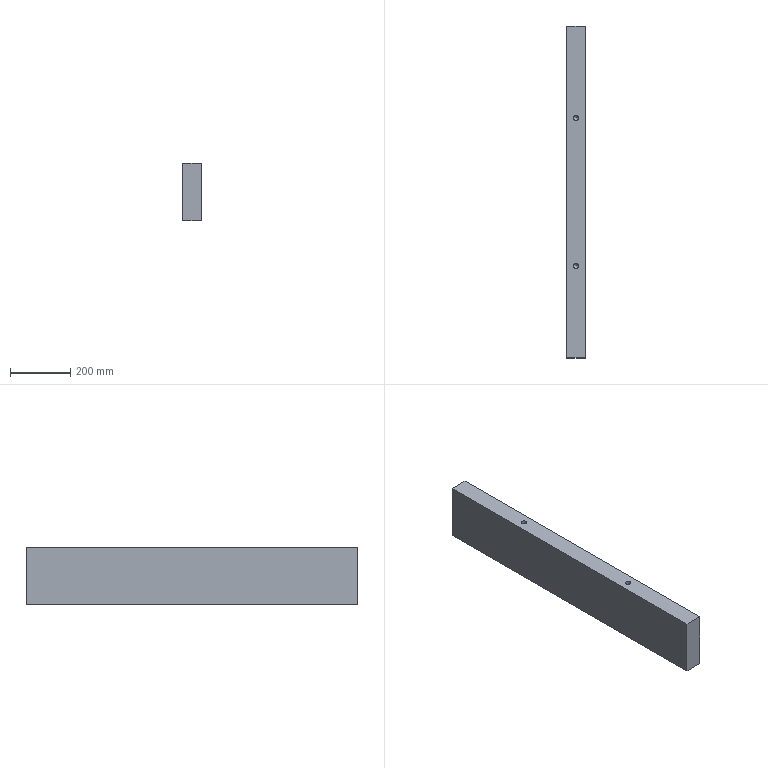Part | STEP file | lll_id4450_x_t | 1 solid | 14 faces | box 60 x 1100 x 190 mm | volume 12497474 mm3 | plane 6 | cylinder 4 | cone 4 | commonest cylinder face diameters 17.506 x4
STEP:
#1=CARTESIAN_POINT('',(2116.188,-465.,-370.));
#2=VERTEX_POINT('',#1);
#3=CARTESIAN_POINT('',(2107.435,-465.,-370.));
#4=DIRECTION('',(0.,0.,1.));
#5=DIRECTION('',(1.,0.,0.));
#6=AXIS2_PLACEMENT_3D('',#3,#4,#5);
#7=CIRCLE('',#6,8.753);
#8=EDGE_CURVE('',#2,#2,#7,.T.);
#9=ORIENTED_EDGE('',*,*,#8,.T.);
#10=EDGE_LOOP('',(#9));
#11=FACE_BOUND('',#10,.T.);
#12=CARTESIAN_POINT('',(2077.435,550.,-370.));
#13=VERTEX_POINT('',#12);
#14=CARTESIAN_POINT('',(2077.435,-550.,-370.));
#15=VERTEX_POINT('',#14);
#16=CARTESIAN_POINT('',(2077.435,1.,-370.));
#17=DIRECTION('',(0.,-1.,0.));
#18=VECTOR('',#17,1.);
#19=LINE('',#16,#18);
#20=EDGE_CURVE('',#13,#15,#19,.T.);
#21=ORIENTED_EDGE('',*,*,#20,.F.);
#22=CARTESIAN_POINT('',(2137.435,550.,-370.));
#23=VERTEX_POINT('',#22);
#24=CARTESIAN_POINT('',(4323.751,550.,-370.));
#25=DIRECTION('',(1.,0.,0.));
#26=VECTOR('',#25,1.);
#27=LINE('',#24,#26);
#28=EDGE_CURVE('',#13,#23,#27,.T.);
#29=ORIENTED_EDGE('',*,*,#28,.T.);
#30=CARTESIAN_POINT('',(2137.435,-550.,-370.));
#31=VERTEX_POINT('',#30);
#32=CARTESIAN_POINT('',(2137.435,600.,-370.));
#33=DIRECTION('',(0.,-1.,0.));
#34=VECTOR('',#33,1.);
#35=LINE('',#32,#34);
#36=EDGE_CURVE('',#23,#31,#35,.T.);
#37=ORIENTED_EDGE('',*,*,#36,.T.);
#38=CARTESIAN_POINT('',(4323.751,-550.,-370.));
#39=DIRECTION('',(-1.,0.,0.));
#40=VECTOR('',#39,1.);
#41=LINE('',#38,#40);
#42=EDGE_CURVE('',#31,#15,#41,.T.);
#43=ORIENTED_EDGE('',*,*,#42,.T.);
#44=EDGE_LOOP('',(#21,#29,#37,#43));
#45=FACE_BOUND('',#44,.T.);
#46=CARTESIAN_POINT('',(2116.188,465.,-370.));
#47=VERTEX_POINT('',#46);
#48=CARTESIAN_POINT('',(2107.435,465.,-370.));
#49=DIRECTION('',(0.,0.,1.));
#50=DIRECTION('',(1.,0.,0.));
#51=AXIS2_PLACEMENT_3D('',#48,#49,#50);
#52=CIRCLE('',#51,8.753);
#53=EDGE_CURVE('',#47,#47,#52,.T.);
#54=ORIENTED_EDGE('',*,*,#53,.T.);
#55=EDGE_LOOP('',(#54));
#56=FACE_BOUND('',#55,.T.);
#57=CARTESIAN_POINT('',(4323.751,1.,-370.));
#58=DIRECTION('',(0.,0.,-1.));
#59=DIRECTION('',(-1.,0.,0.));
#60=AXIS2_PLACEMENT_3D('',#57,#58,#59);
#61=PLANE('',#60);
#62=ADVANCED_FACE('',(#11,#45,#56),#61,.T.);
#63=ORIENTED_EDGE('',*,*,#36,.F.);
#64=CARTESIAN_POINT('',(2137.435,550.,-180.));
#65=VERTEX_POINT('',#64);
#66=CARTESIAN_POINT('',(2137.435,550.,-182.5));
#67=DIRECTION('',(0.,0.,-1.));
#68=VECTOR('',#67,1.);
#69=LINE('',#66,#68);
#70=EDGE_CURVE('',#65,#23,#69,.T.);
#71=ORIENTED_EDGE('',*,*,#70,.F.);
#72=CARTESIAN_POINT('',(2137.435,-550.,-180.));
#73=VERTEX_POINT('',#72);
#74=CARTESIAN_POINT('',(2137.435,1.,-180.));
#75=DIRECTION('',(0.,-1.,0.));
#76=VECTOR('',#75,1.);
#77=LINE('',#74,#76);
#78=EDGE_CURVE('',#65,#73,#77,.T.);
#79=ORIENTED_EDGE('',*,*,#78,.T.);
#80=CARTESIAN_POINT('',(2137.435,-550.,-182.5));
#81=DIRECTION('',(0.,0.,-1.));
#82=VECTOR('',#81,1.);
#83=LINE('',#80,#82);
#84=EDGE_CURVE('',#73,#31,#83,.T.);
#85=ORIENTED_EDGE('',*,*,#84,.T.);
#86=EDGE_LOOP('',(#63,#71,#79,#85));
#87=FACE_OUTER_BOUND('',#86,.T.);
#88=CARTESIAN_POINT('',(2137.435,600.,-182.5));
#89=DIRECTION('',(1.,0.,0.));
#90=DIRECTION('',(0.,0.,-1.));
#91=AXIS2_PLACEMENT_3D('',#88,#89,#90);
#92=PLANE('',#91);
#93=ADVANCED_FACE('',(#87),#92,.T.);
#94=CARTESIAN_POINT('',(2077.435,-550.,-180.));
#95=VERTEX_POINT('',#94);
#96=CARTESIAN_POINT('',(2077.435,-550.,-251.25));
#97=DIRECTION('',(0.,0.,-1.));
#98=VECTOR('',#97,1.);
#99=LINE('',#96,#98);
#100=EDGE_CURVE('',#95,#15,#99,.T.);
#101=ORIENTED_EDGE('',*,*,#100,.T.);
#102=ORIENTED_EDGE('',*,*,#42,.F.);
#103=ORIENTED_EDGE('',*,*,#84,.F.);
#104=CARTESIAN_POINT('',(4323.751,-550.,-180.));
#105=DIRECTION('',(-1.,0.,0.));
#106=VECTOR('',#105,1.);
#107=LINE('',#104,#106);
#108=EDGE_CURVE('',#73,#95,#107,.T.);
#109=ORIENTED_EDGE('',*,*,#108,.T.);
#110=EDGE_LOOP('',(#101,#102,#103,#109));
#111=FACE_OUTER_BOUND('',#110,.T.);
#112=CARTESIAN_POINT('',(2137.435,-550.,-182.5));
#113=DIRECTION('',(0.,-1.,0.));
#114=DIRECTION('',(0.,0.,-1.));
#115=AXIS2_PLACEMENT_3D('',#112,#113,#114);
#116=PLANE('',#115);
#117=ADVANCED_FACE('',(#111),#116,.T.);
#118=CARTESIAN_POINT('',(2077.435,550.,-180.));
#119=VERTEX_POINT('',#118);
#120=CARTESIAN_POINT('',(2077.435,550.,-251.25));
#121=DIRECTION('',(0.,0.,1.));
#122=VECTOR('',#121,1.);
#123=LINE('',#120,#122);
#124=EDGE_CURVE('',#13,#119,#123,.T.);
#125=ORIENTED_EDGE('',*,*,#124,.T.);
#126=CARTESIAN_POINT('',(4323.751,550.,-180.));
#127=DIRECTION('',(1.,0.,0.));
#128=VECTOR('',#127,1.);
#129=LINE('',#126,#128);
#130=EDGE_CURVE('',#119,#65,#129,.T.);
#131=ORIENTED_EDGE('',*,*,#130,.T.);
#132=ORIENTED_EDGE('',*,*,#70,.T.);
#133=ORIENTED_EDGE('',*,*,#28,.F.);
#134=EDGE_LOOP('',(#125,#131,#132,#133));
#135=FACE_OUTER_BOUND('',#134,.T.);
#136=CARTESIAN_POINT('',(-1832.565,550.,-182.5));
#137=DIRECTION('',(0.,1.,0.));
#138=DIRECTION('',(0.,0.,1.));
#139=AXIS2_PLACEMENT_3D('',#136,#137,#138);
#140=PLANE('',#139);
#141=ADVANCED_FACE('',(#135),#140,.T.);
#142=CARTESIAN_POINT('',(2098.682,245.,-180.));
#143=VERTEX_POINT('',#142);
#144=CARTESIAN_POINT('',(2107.435,245.,-180.));
#145=DIRECTION('',(0.,0.,-1.));
#146=DIRECTION('',(-1.,0.,0.));
#147=AXIS2_PLACEMENT_3D('',#144,#145,#146);
#148=CIRCLE('',#147,8.753);
#149=EDGE_CURVE('',#143,#143,#148,.T.);
#150=ORIENTED_EDGE('',*,*,#149,.T.);
#151=EDGE_LOOP('',(#150));
#152=FACE_BOUND('',#151,.T.);
#153=CARTESIAN_POINT('',(2098.682,-245.,-180.));
#154=VERTEX_POINT('',#153);
#155=CARTESIAN_POINT('',(2107.435,-245.,-180.));
#156=DIRECTION('',(0.,0.,-1.));
#157=DIRECTION('',(-1.,0.,0.));
#158=AXIS2_PLACEMENT_3D('',#155,#156,#157);
#159=CIRCLE('',#158,8.753);
#160=EDGE_CURVE('',#154,#154,#159,.T.);
#161=ORIENTED_EDGE('',*,*,#160,.T.);
#162=EDGE_LOOP('',(#161));
#163=FACE_BOUND('',#162,.T.);
#164=ORIENTED_EDGE('',*,*,#130,.F.);
#165=CARTESIAN_POINT('',(2077.435,0.,-180.));
#166=DIRECTION('',(0.,1.,0.));
#167=VECTOR('',#166,1.);
#168=LINE('',#165,#167);
#169=EDGE_CURVE('',#95,#119,#168,.T.);
#170=ORIENTED_EDGE('',*,*,#169,.F.);
#171=ORIENTED_EDGE('',*,*,#108,.F.);
#172=ORIENTED_EDGE('',*,*,#78,.F.);
#173=EDGE_LOOP('',(#164,#170,#171,#172));
#174=FACE_BOUND('',#173,.T.);
#175=CARTESIAN_POINT('',(4323.751,1.,-180.));
#176=DIRECTION('',(0.,0.,-1.));
#177=DIRECTION('',(-1.,0.,0.));
#178=AXIS2_PLACEMENT_3D('',#175,#176,#177);
#179=PLANE('',#178);
#180=ADVANCED_FACE('',(#152,#163,#174),#179,.F.);
#181=ORIENTED_EDGE('',*,*,#124,.F.);
#182=ORIENTED_EDGE('',*,*,#20,.T.);
#183=ORIENTED_EDGE('',*,*,#100,.F.);
#184=ORIENTED_EDGE('',*,*,#169,.T.);
#185=EDGE_LOOP('',(#181,#182,#183,#184));
#186=FACE_OUTER_BOUND('',#185,.T.);
#187=CARTESIAN_POINT('',(2077.435,0.,-251.25));
#188=DIRECTION('',(1.,0.,0.));
#189=DIRECTION('',(0.,0.,-1.));
#190=AXIS2_PLACEMENT_3D('',#187,#188,#189);
#191=PLANE('',#190);
#192=ADVANCED_FACE('',(#186),#191,.F.);
#193=CARTESIAN_POINT('',(2116.188,-465.,-328.747));
#194=VERTEX_POINT('',#193);
#195=CARTESIAN_POINT('',(2107.435,-465.,-328.747));
#196=DIRECTION('',(0.,0.,1.));
#197=DIRECTION('',(1.,0.,0.));
#198=AXIS2_PLACEMENT_3D('',#195,#196,#197);
#199=CIRCLE('',#198,8.753);
#200=EDGE_CURVE('',#194,#194,#199,.T.);
#201=ORIENTED_EDGE('',*,*,#200,.T.);
#202=EDGE_LOOP('',(#201));
#203=FACE_BOUND('',#202,.T.);
#204=ORIENTED_EDGE('',*,*,#8,.F.);
#205=EDGE_LOOP('',(#204));
#206=FACE_BOUND('',#205,.T.);
#207=CARTESIAN_POINT('',(2107.435,-465.,-370.));
#208=DIRECTION('',(0.,0.,1.));
#209=DIRECTION('',(-1.,0.,0.));
#210=AXIS2_PLACEMENT_3D('',#207,#208,#209);
#211=CYLINDRICAL_SURFACE('',#210,8.753);
#212=ADVANCED_FACE('',(#203,#206),#211,.F.);
#213=CARTESIAN_POINT('',(2107.435,-465.,-319.994));
#214=VERTEX_POINT('',#213);
#215=VERTEX_LOOP('',#214);
#216=FACE_BOUND('',#215,.T.);
#217=ORIENTED_EDGE('',*,*,#200,.F.);
#218=EDGE_LOOP('',(#217));
#219=FACE_BOUND('',#218,.T.);
#220=CARTESIAN_POINT('',(2107.435,-465.,-328.747));
#221=DIRECTION('',(0.,0.,-1.));
#222=DIRECTION('',(1.,0.,0.));
#223=AXIS2_PLACEMENT_3D('',#220,#221,#222);
#224=CONICAL_SURFACE('',#223,8.753,45.);
#225=ADVANCED_FACE('',(#216,#219),#224,.F.);
#226=CARTESIAN_POINT('',(2116.188,465.,-328.747));
#227=VERTEX_POINT('',#226);
#228=CARTESIAN_POINT('',(2107.435,465.,-328.747));
#229=DIRECTION('',(0.,0.,1.));
#230=DIRECTION('',(1.,0.,0.));
#231=AXIS2_PLACEMENT_3D('',#228,#229,#230);
#232=CIRCLE('',#231,8.753);
#233=EDGE_CURVE('',#227,#227,#232,.T.);
#234=ORIENTED_EDGE('',*,*,#233,.T.);
#235=EDGE_LOOP('',(#234));
#236=FACE_BOUND('',#235,.T.);
#237=ORIENTED_EDGE('',*,*,#53,.F.);
#238=EDGE_LOOP('',(#237));
#239=FACE_BOUND('',#238,.T.);
#240=CARTESIAN_POINT('',(2107.435,465.,-370.));
#241=DIRECTION('',(0.,0.,1.));
#242=DIRECTION('',(-1.,0.,0.));
#243=AXIS2_PLACEMENT_3D('',#240,#241,#242);
#244=CYLINDRICAL_SURFACE('',#243,8.753);
#245=ADVANCED_FACE('',(#236,#239),#244,.F.);
#246=CARTESIAN_POINT('',(2107.435,465.,-319.994));
#247=VERTEX_POINT('',#246);
#248=VERTEX_LOOP('',#247);
#249=FACE_BOUND('',#248,.T.);
#250=ORIENTED_EDGE('',*,*,#233,.F.);
#251=EDGE_LOOP('',(#250));
#252=FACE_BOUND('',#251,.T.);
#253=CARTESIAN_POINT('',(2107.435,465.,-328.747));
#254=DIRECTION('',(0.,0.,-1.));
#255=DIRECTION('',(1.,0.,0.));
#256=AXIS2_PLACEMENT_3D('',#253,#254,#255);
#257=CONICAL_SURFACE('',#256,8.753,45.);
#258=ADVANCED_FACE('',(#249,#252),#257,.F.);
#259=CARTESIAN_POINT('',(2098.682,-245.,-221.253));
#260=VERTEX_POINT('',#259);
#261=CARTESIAN_POINT('',(2107.435,-245.,-221.253));
#262=DIRECTION('',(0.,0.,-1.));
#263=DIRECTION('',(-1.,0.,0.));
#264=AXIS2_PLACEMENT_3D('',#261,#262,#263);
#265=CIRCLE('',#264,8.753);
#266=EDGE_CURVE('',#260,#260,#265,.T.);
#267=ORIENTED_EDGE('',*,*,#266,.T.);
#268=EDGE_LOOP('',(#267));
#269=FACE_BOUND('',#268,.T.);
#270=ORIENTED_EDGE('',*,*,#160,.F.);
#271=EDGE_LOOP('',(#270));
#272=FACE_BOUND('',#271,.T.);
#273=CARTESIAN_POINT('',(2107.435,-245.,-180.));
#274=DIRECTION('',(0.,0.,-1.));
#275=DIRECTION('',(1.,0.,0.));
#276=AXIS2_PLACEMENT_3D('',#273,#274,#275);
#277=CYLINDRICAL_SURFACE('',#276,8.753);
#278=ADVANCED_FACE('',(#269,#272),#277,.F.);
#279=CARTESIAN_POINT('',(2107.435,-245.,-230.006));
#280=VERTEX_POINT('',#279);
#281=VERTEX_LOOP('',#280);
#282=FACE_BOUND('',#281,.T.);
#283=ORIENTED_EDGE('',*,*,#266,.F.);
#284=EDGE_LOOP('',(#283));
#285=FACE_BOUND('',#284,.T.);
#286=CARTESIAN_POINT('',(2107.435,-245.,-221.253));
#287=DIRECTION('',(0.,0.,1.));
#288=DIRECTION('',(-1.,0.,0.));
#289=AXIS2_PLACEMENT_3D('',#286,#287,#288);
#290=CONICAL_SURFACE('',#289,8.753,45.);
#291=ADVANCED_FACE('',(#282,#285),#290,.F.);
#292=CARTESIAN_POINT('',(2098.682,245.,-221.253));
#293=VERTEX_POINT('',#292);
#294=CARTESIAN_POINT('',(2107.435,245.,-221.253));
#295=DIRECTION('',(0.,0.,-1.));
#296=DIRECTION('',(-1.,0.,0.));
#297=AXIS2_PLACEMENT_3D('',#294,#295,#296);
#298=CIRCLE('',#297,8.753);
#299=EDGE_CURVE('',#293,#293,#298,.T.);
#300=ORIENTED_EDGE('',*,*,#299,.T.);
#301=EDGE_LOOP('',(#300));
#302=FACE_BOUND('',#301,.T.);
#303=ORIENTED_EDGE('',*,*,#149,.F.);
#304=EDGE_LOOP('',(#303));
#305=FACE_BOUND('',#304,.T.);
#306=CARTESIAN_POINT('',(2107.435,245.,-180.));
#307=DIRECTION('',(0.,0.,-1.));
#308=DIRECTION('',(1.,0.,0.));
#309=AXIS2_PLACEMENT_3D('',#306,#307,#308);
#310=CYLINDRICAL_SURFACE('',#309,8.753);
#311=ADVANCED_FACE('',(#302,#305),#310,.F.);
#312=CARTESIAN_POINT('',(2107.435,245.,-230.006));
#313=VERTEX_POINT('',#312);
#314=VERTEX_LOOP('',#313);
#315=FACE_BOUND('',#314,.T.);
#316=ORIENTED_EDGE('',*,*,#299,.F.);
#317=EDGE_LOOP('',(#316));
#318=FACE_BOUND('',#317,.T.);
#319=CARTESIAN_POINT('',(2107.435,245.,-221.253));
#320=DIRECTION('',(0.,0.,1.));
#321=DIRECTION('',(-1.,0.,0.));
#322=AXIS2_PLACEMENT_3D('',#319,#320,#321);
#323=CONICAL_SURFACE('',#322,8.753,45.);
#324=ADVANCED_FACE('',(#315,#318),#323,.F.);
#325=CLOSED_SHELL('',(#62,#93,#117,#141,#180,#192,#212,#225,#245,#258,#278,#291,#311,#324));
#326=MANIFOLD_SOLID_BREP('',#325);
#327=(LENGTH_UNIT()NAMED_UNIT(*)SI_UNIT(.MILLI.,.METRE.));
#328=UNCERTAINTY_MEASURE_WITH_UNIT(LENGTH_MEASURE(0.00002),#327,'','');
#329=(NAMED_UNIT(*)PLANE_ANGLE_UNIT()SI_UNIT($,.RADIAN.));
#330=PLANE_ANGLE_MEASURE_WITH_UNIT(PLANE_ANGLE_MEASURE(0.01745),#329);
#331=DIMENSIONAL_EXPONENTS(0.,0.,0.,0.,0.,0.,0.);
#332=(CONVERSION_BASED_UNIT('DEGREE',#330)NAMED_UNIT(#331)PLANE_ANGLE_UNIT());
#333=(NAMED_UNIT(*)SI_UNIT($,.STERADIAN.)SOLID_ANGLE_UNIT());
#334=(GEOMETRIC_REPRESENTATION_CONTEXT(3)GLOBAL_UNCERTAINTY_ASSIGNED_CONTEXT((#328))GLOBAL_UNIT_ASSIGNED_CONTEXT((#327,#332,#333))REPRESENTATION_CONTEXT('',''));
#335=ADVANCED_BREP_SHAPE_REPRESENTATION('',(#326),#334);